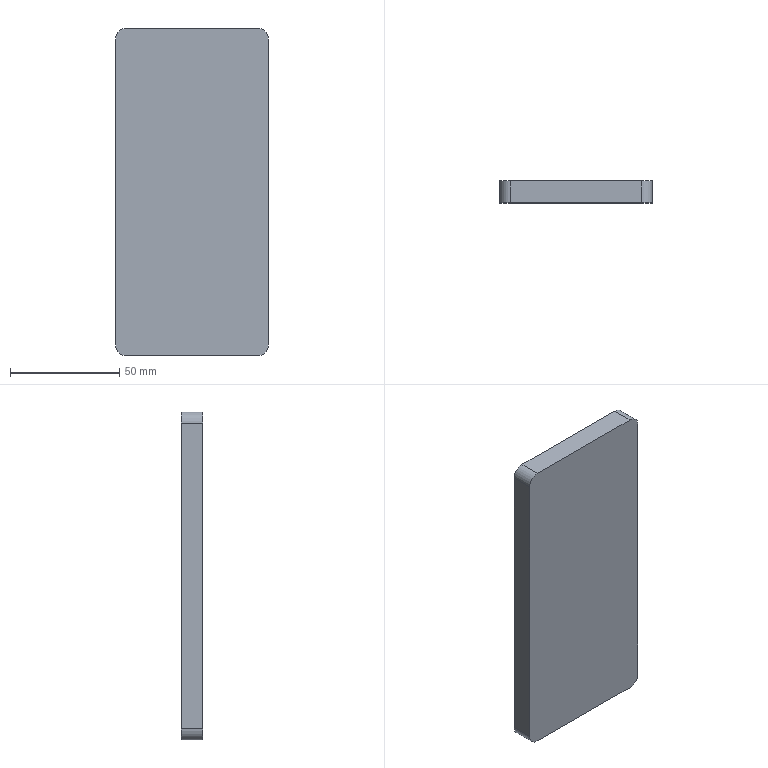Part | SolidWorks | features BaseBody 1 | 1 solid | 10 faces | box 70 x 10 x 150 mm | volume 104785 mm3 | plane 6 | cylinder 4 | commonest cylinder face diameters 10 x4
STEP:
#1=CARTESIAN_POINT('',(-35.,-5.,70.));
#2=VERTEX_POINT('',#1);
#3=CARTESIAN_POINT('',(-30.,-5.,75.));
#4=VERTEX_POINT('',#3);
#5=CARTESIAN_POINT('',(-30.,-5.,70.));
#6=DIRECTION('',(0.,1.,0.));
#7=DIRECTION('',(0.,0.,1.));
#8=AXIS2_PLACEMENT_3D('',#5,#6,#7);
#9=CIRCLE('',#8,5.);
#10=EDGE_CURVE('',#2,#4,#9,.T.);
#11=ORIENTED_EDGE('',*,*,#10,.T.);
#12=CARTESIAN_POINT('',(-30.,5.,75.));
#13=VERTEX_POINT('',#12);
#14=CARTESIAN_POINT('',(-30.,5.,75.));
#15=DIRECTION('',(0.,-1.,0.));
#16=VECTOR('',#15,1000.);
#17=LINE('',#14,#16);
#18=EDGE_CURVE('',#13,#4,#17,.T.);
#19=ORIENTED_EDGE('',*,*,#18,.F.);
#20=CARTESIAN_POINT('',(-35.,5.,70.));
#21=VERTEX_POINT('',#20);
#22=CARTESIAN_POINT('',(-30.,5.,70.));
#23=DIRECTION('',(0.,1.,0.));
#24=DIRECTION('',(0.,0.,1.));
#25=AXIS2_PLACEMENT_3D('',#22,#23,#24);
#26=CIRCLE('',#25,5.);
#27=EDGE_CURVE('',#21,#13,#26,.T.);
#28=ORIENTED_EDGE('',*,*,#27,.F.);
#29=CARTESIAN_POINT('',(-35.,5.,70.));
#30=DIRECTION('',(0.,-1.,0.));
#31=VECTOR('',#30,1000.);
#32=LINE('',#29,#31);
#33=EDGE_CURVE('',#21,#2,#32,.T.);
#34=ORIENTED_EDGE('',*,*,#33,.T.);
#35=EDGE_LOOP('',(#11,#19,#28,#34));
#36=FACE_OUTER_BOUND('',#35,.T.);
#37=CARTESIAN_POINT('',(-30.,5.,70.));
#38=DIRECTION('',(0.,-1.,0.));
#39=DIRECTION('',(0.,0.,-1.));
#40=AXIS2_PLACEMENT_3D('',#37,#38,#39);
#41=CYLINDRICAL_SURFACE('',#40,5.);
#42=ADVANCED_FACE('',(#36),#41,.T.);
#43=CARTESIAN_POINT('',(30.,-5.,75.));
#44=VERTEX_POINT('',#43);
#45=CARTESIAN_POINT('',(-30.,-5.,75.));
#46=DIRECTION('',(1.,0.,0.));
#47=VECTOR('',#46,1000.);
#48=LINE('',#45,#47);
#49=EDGE_CURVE('',#4,#44,#48,.T.);
#50=ORIENTED_EDGE('',*,*,#49,.T.);
#51=CARTESIAN_POINT('',(30.,5.,75.));
#52=VERTEX_POINT('',#51);
#53=CARTESIAN_POINT('',(30.,5.,75.));
#54=DIRECTION('',(0.,-1.,0.));
#55=VECTOR('',#54,1000.);
#56=LINE('',#53,#55);
#57=EDGE_CURVE('',#52,#44,#56,.T.);
#58=ORIENTED_EDGE('',*,*,#57,.F.);
#59=CARTESIAN_POINT('',(-30.,5.,75.));
#60=DIRECTION('',(1.,0.,0.));
#61=VECTOR('',#60,1000.);
#62=LINE('',#59,#61);
#63=EDGE_CURVE('',#13,#52,#62,.T.);
#64=ORIENTED_EDGE('',*,*,#63,.F.);
#65=ORIENTED_EDGE('',*,*,#18,.T.);
#66=EDGE_LOOP('',(#50,#58,#64,#65));
#67=FACE_OUTER_BOUND('',#66,.T.);
#68=CARTESIAN_POINT('',(-30.,5.,75.));
#69=DIRECTION('',(0.,0.,-1.));
#70=DIRECTION('',(-1.,0.,0.));
#71=AXIS2_PLACEMENT_3D('',#68,#69,#70);
#72=PLANE('',#71);
#73=ADVANCED_FACE('',(#67),#72,.F.);
#74=CARTESIAN_POINT('',(35.,-5.,70.));
#75=VERTEX_POINT('',#74);
#76=CARTESIAN_POINT('',(30.,-5.,70.));
#77=DIRECTION('',(0.,1.,0.));
#78=DIRECTION('',(0.,0.,1.));
#79=AXIS2_PLACEMENT_3D('',#76,#77,#78);
#80=CIRCLE('',#79,5.);
#81=EDGE_CURVE('',#44,#75,#80,.T.);
#82=ORIENTED_EDGE('',*,*,#81,.T.);
#83=CARTESIAN_POINT('',(35.,5.,70.));
#84=VERTEX_POINT('',#83);
#85=CARTESIAN_POINT('',(35.,5.,70.));
#86=DIRECTION('',(0.,-1.,0.));
#87=VECTOR('',#86,1000.);
#88=LINE('',#85,#87);
#89=EDGE_CURVE('',#84,#75,#88,.T.);
#90=ORIENTED_EDGE('',*,*,#89,.F.);
#91=CARTESIAN_POINT('',(30.,5.,70.));
#92=DIRECTION('',(0.,1.,0.));
#93=DIRECTION('',(0.,0.,1.));
#94=AXIS2_PLACEMENT_3D('',#91,#92,#93);
#95=CIRCLE('',#94,5.);
#96=EDGE_CURVE('',#52,#84,#95,.T.);
#97=ORIENTED_EDGE('',*,*,#96,.F.);
#98=ORIENTED_EDGE('',*,*,#57,.T.);
#99=EDGE_LOOP('',(#82,#90,#97,#98));
#100=FACE_OUTER_BOUND('',#99,.T.);
#101=CARTESIAN_POINT('',(30.,5.,70.));
#102=DIRECTION('',(0.,-1.,0.));
#103=DIRECTION('',(0.,0.,-1.));
#104=AXIS2_PLACEMENT_3D('',#101,#102,#103);
#105=CYLINDRICAL_SURFACE('',#104,5.);
#106=ADVANCED_FACE('',(#100),#105,.T.);
#107=CARTESIAN_POINT('',(35.,-5.,-70.));
#108=VERTEX_POINT('',#107);
#109=CARTESIAN_POINT('',(35.,-5.,-70.));
#110=DIRECTION('',(0.,0.,-1.));
#111=VECTOR('',#110,1000.);
#112=LINE('',#109,#111);
#113=EDGE_CURVE('',#75,#108,#112,.T.);
#114=ORIENTED_EDGE('',*,*,#113,.T.);
#115=CARTESIAN_POINT('',(35.,5.,-70.));
#116=VERTEX_POINT('',#115);
#117=CARTESIAN_POINT('',(35.,5.,-70.));
#118=DIRECTION('',(0.,-1.,0.));
#119=VECTOR('',#118,1000.);
#120=LINE('',#117,#119);
#121=EDGE_CURVE('',#116,#108,#120,.T.);
#122=ORIENTED_EDGE('',*,*,#121,.F.);
#123=CARTESIAN_POINT('',(35.,5.,-70.));
#124=DIRECTION('',(0.,0.,-1.));
#125=VECTOR('',#124,1000.);
#126=LINE('',#123,#125);
#127=EDGE_CURVE('',#84,#116,#126,.T.);
#128=ORIENTED_EDGE('',*,*,#127,.F.);
#129=ORIENTED_EDGE('',*,*,#89,.T.);
#130=EDGE_LOOP('',(#114,#122,#128,#129));
#131=FACE_OUTER_BOUND('',#130,.T.);
#132=CARTESIAN_POINT('',(35.,5.,-70.));
#133=DIRECTION('',(-1.,0.,0.));
#134=DIRECTION('',(0.,0.,1.));
#135=AXIS2_PLACEMENT_3D('',#132,#133,#134);
#136=PLANE('',#135);
#137=ADVANCED_FACE('',(#131),#136,.F.);
#138=CARTESIAN_POINT('',(30.,-5.,-75.));
#139=VERTEX_POINT('',#138);
#140=CARTESIAN_POINT('',(30.,-5.,-70.));
#141=DIRECTION('',(0.,1.,0.));
#142=DIRECTION('',(0.,0.,-1.));
#143=AXIS2_PLACEMENT_3D('',#140,#141,#142);
#144=CIRCLE('',#143,5.);
#145=EDGE_CURVE('',#108,#139,#144,.T.);
#146=ORIENTED_EDGE('',*,*,#145,.T.);
#147=CARTESIAN_POINT('',(30.,5.,-75.));
#148=VERTEX_POINT('',#147);
#149=CARTESIAN_POINT('',(30.,5.,-75.));
#150=DIRECTION('',(0.,-1.,0.));
#151=VECTOR('',#150,1000.);
#152=LINE('',#149,#151);
#153=EDGE_CURVE('',#148,#139,#152,.T.);
#154=ORIENTED_EDGE('',*,*,#153,.F.);
#155=CARTESIAN_POINT('',(30.,5.,-70.));
#156=DIRECTION('',(0.,1.,0.));
#157=DIRECTION('',(0.,0.,-1.));
#158=AXIS2_PLACEMENT_3D('',#155,#156,#157);
#159=CIRCLE('',#158,5.);
#160=EDGE_CURVE('',#116,#148,#159,.T.);
#161=ORIENTED_EDGE('',*,*,#160,.F.);
#162=ORIENTED_EDGE('',*,*,#121,.T.);
#163=EDGE_LOOP('',(#146,#154,#161,#162));
#164=FACE_OUTER_BOUND('',#163,.T.);
#165=CARTESIAN_POINT('',(30.,5.,-70.));
#166=DIRECTION('',(0.,-1.,0.));
#167=DIRECTION('',(0.,0.,-1.));
#168=AXIS2_PLACEMENT_3D('',#165,#166,#167);
#169=CYLINDRICAL_SURFACE('',#168,5.);
#170=ADVANCED_FACE('',(#164),#169,.T.);
#171=CARTESIAN_POINT('',(-30.,-5.,-75.));
#172=VERTEX_POINT('',#171);
#173=CARTESIAN_POINT('',(-30.,-5.,-75.));
#174=DIRECTION('',(-1.,0.,0.));
#175=VECTOR('',#174,1000.);
#176=LINE('',#173,#175);
#177=EDGE_CURVE('',#139,#172,#176,.T.);
#178=ORIENTED_EDGE('',*,*,#177,.T.);
#179=CARTESIAN_POINT('',(-30.,5.,-75.));
#180=VERTEX_POINT('',#179);
#181=CARTESIAN_POINT('',(-30.,5.,-75.));
#182=DIRECTION('',(0.,-1.,0.));
#183=VECTOR('',#182,1000.);
#184=LINE('',#181,#183);
#185=EDGE_CURVE('',#180,#172,#184,.T.);
#186=ORIENTED_EDGE('',*,*,#185,.F.);
#187=CARTESIAN_POINT('',(-30.,5.,-75.));
#188=DIRECTION('',(-1.,0.,0.));
#189=VECTOR('',#188,1000.);
#190=LINE('',#187,#189);
#191=EDGE_CURVE('',#148,#180,#190,.T.);
#192=ORIENTED_EDGE('',*,*,#191,.F.);
#193=ORIENTED_EDGE('',*,*,#153,.T.);
#194=EDGE_LOOP('',(#178,#186,#192,#193));
#195=FACE_OUTER_BOUND('',#194,.T.);
#196=CARTESIAN_POINT('',(-30.,5.,-75.));
#197=DIRECTION('',(0.,0.,1.));
#198=DIRECTION('',(1.,0.,0.));
#199=AXIS2_PLACEMENT_3D('',#196,#197,#198);
#200=PLANE('',#199);
#201=ADVANCED_FACE('',(#195),#200,.F.);
#202=CARTESIAN_POINT('',(-35.,-5.,-70.));
#203=VERTEX_POINT('',#202);
#204=CARTESIAN_POINT('',(-30.,-5.,-70.));
#205=DIRECTION('',(0.,1.,0.));
#206=DIRECTION('',(0.,0.,1.));
#207=AXIS2_PLACEMENT_3D('',#204,#205,#206);
#208=CIRCLE('',#207,5.);
#209=EDGE_CURVE('',#172,#203,#208,.T.);
#210=ORIENTED_EDGE('',*,*,#209,.T.);
#211=CARTESIAN_POINT('',(-35.,5.,-70.));
#212=VERTEX_POINT('',#211);
#213=CARTESIAN_POINT('',(-35.,5.,-70.));
#214=DIRECTION('',(0.,-1.,0.));
#215=VECTOR('',#214,1000.);
#216=LINE('',#213,#215);
#217=EDGE_CURVE('',#212,#203,#216,.T.);
#218=ORIENTED_EDGE('',*,*,#217,.F.);
#219=CARTESIAN_POINT('',(-30.,5.,-70.));
#220=DIRECTION('',(0.,1.,0.));
#221=DIRECTION('',(0.,0.,1.));
#222=AXIS2_PLACEMENT_3D('',#219,#220,#221);
#223=CIRCLE('',#222,5.);
#224=EDGE_CURVE('',#180,#212,#223,.T.);
#225=ORIENTED_EDGE('',*,*,#224,.F.);
#226=ORIENTED_EDGE('',*,*,#185,.T.);
#227=EDGE_LOOP('',(#210,#218,#225,#226));
#228=FACE_OUTER_BOUND('',#227,.T.);
#229=CARTESIAN_POINT('',(-30.,5.,-70.));
#230=DIRECTION('',(0.,-1.,0.));
#231=DIRECTION('',(0.,0.,-1.));
#232=AXIS2_PLACEMENT_3D('',#229,#230,#231);
#233=CYLINDRICAL_SURFACE('',#232,5.);
#234=ADVANCED_FACE('',(#228),#233,.T.);
#235=CARTESIAN_POINT('',(-35.,-5.,-70.));
#236=DIRECTION('',(0.,0.,1.));
#237=VECTOR('',#236,1000.);
#238=LINE('',#235,#237);
#239=EDGE_CURVE('',#203,#2,#238,.T.);
#240=ORIENTED_EDGE('',*,*,#239,.T.);
#241=ORIENTED_EDGE('',*,*,#33,.F.);
#242=CARTESIAN_POINT('',(-35.,5.,-70.));
#243=DIRECTION('',(0.,0.,1.));
#244=VECTOR('',#243,1000.);
#245=LINE('',#242,#244);
#246=EDGE_CURVE('',#212,#21,#245,.T.);
#247=ORIENTED_EDGE('',*,*,#246,.F.);
#248=ORIENTED_EDGE('',*,*,#217,.T.);
#249=EDGE_LOOP('',(#240,#241,#247,#248));
#250=FACE_OUTER_BOUND('',#249,.T.);
#251=CARTESIAN_POINT('',(-35.,5.,-70.));
#252=DIRECTION('',(1.,0.,0.));
#253=DIRECTION('',(0.,0.,-1.));
#254=AXIS2_PLACEMENT_3D('',#251,#252,#253);
#255=PLANE('',#254);
#256=ADVANCED_FACE('',(#250),#255,.F.);
#257=ORIENTED_EDGE('',*,*,#27,.T.);
#258=ORIENTED_EDGE('',*,*,#63,.T.);
#259=ORIENTED_EDGE('',*,*,#96,.T.);
#260=ORIENTED_EDGE('',*,*,#127,.T.);
#261=ORIENTED_EDGE('',*,*,#160,.T.);
#262=ORIENTED_EDGE('',*,*,#191,.T.);
#263=ORIENTED_EDGE('',*,*,#224,.T.);
#264=ORIENTED_EDGE('',*,*,#246,.T.);
#265=EDGE_LOOP('',(#257,#258,#259,#260,#261,#262,#263,#264));
#266=FACE_OUTER_BOUND('',#265,.T.);
#267=CARTESIAN_POINT('',(-30.,5.,70.));
#268=DIRECTION('',(0.,1.,0.));
#269=DIRECTION('',(0.,0.,1.));
#270=AXIS2_PLACEMENT_3D('',#267,#268,#269);
#271=PLANE('',#270);
#272=ADVANCED_FACE('',(#266),#271,.T.);
#273=ORIENTED_EDGE('',*,*,#10,.F.);
#274=ORIENTED_EDGE('',*,*,#239,.F.);
#275=ORIENTED_EDGE('',*,*,#209,.F.);
#276=ORIENTED_EDGE('',*,*,#177,.F.);
#277=ORIENTED_EDGE('',*,*,#145,.F.);
#278=ORIENTED_EDGE('',*,*,#113,.F.);
#279=ORIENTED_EDGE('',*,*,#81,.F.);
#280=ORIENTED_EDGE('',*,*,#49,.F.);
#281=EDGE_LOOP('',(#273,#274,#275,#276,#277,#278,#279,#280));
#282=FACE_OUTER_BOUND('',#281,.T.);
#283=CARTESIAN_POINT('',(-30.,-5.,70.));
#284=DIRECTION('',(0.,1.,0.));
#285=DIRECTION('',(0.,0.,1.));
#286=AXIS2_PLACEMENT_3D('',#283,#284,#285);
#287=PLANE('',#286);
#288=ADVANCED_FACE('',(#282),#287,.F.);
#289=CLOSED_SHELL('',(#42,#73,#106,#137,#170,#201,#234,#256,#272,#288));
#290=MANIFOLD_SOLID_BREP('',#289);
#291=CARTESIAN_POINT('',(0.,0.,0.));
#292=DIRECTION('',(0.,0.,1.));
#293=DIRECTION('',(1.,0.,0.));
#294=AXIS2_PLACEMENT_3D('',#291,#292,#293);
#295=(LENGTH_UNIT()NAMED_UNIT(*)SI_UNIT(.MILLI.,.METRE.));
#296=UNCERTAINTY_MEASURE_WITH_UNIT(LENGTH_MEASURE(0.00001),#295,'','');
#297=(NAMED_UNIT(*)PLANE_ANGLE_UNIT()SI_UNIT($,.RADIAN.));
#298=(NAMED_UNIT(*)SI_UNIT($,.STERADIAN.)SOLID_ANGLE_UNIT());
#299=(GEOMETRIC_REPRESENTATION_CONTEXT(3)GLOBAL_UNCERTAINTY_ASSIGNED_CONTEXT((#296))GLOBAL_UNIT_ASSIGNED_CONTEXT((#295,#297,#298))REPRESENTATION_CONTEXT('',''));
#300=ADVANCED_BREP_SHAPE_REPRESENTATION('',(#290,#294),#299);